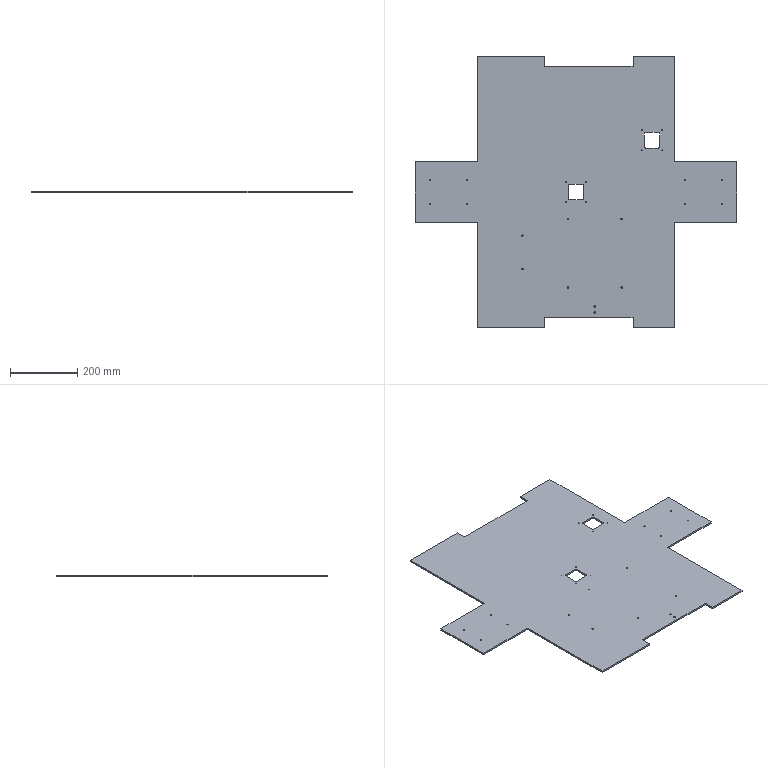Part | NX | features BREP 1 | 1 solid | 62 faces | box 960 x 810 x 5 mm | volume 2619933 mm3 | cylinder 32 | plane 30 | commonest cylinder face diameters 2.5 x8 3.4 x8 10 x8 4.3 x6 5 x2